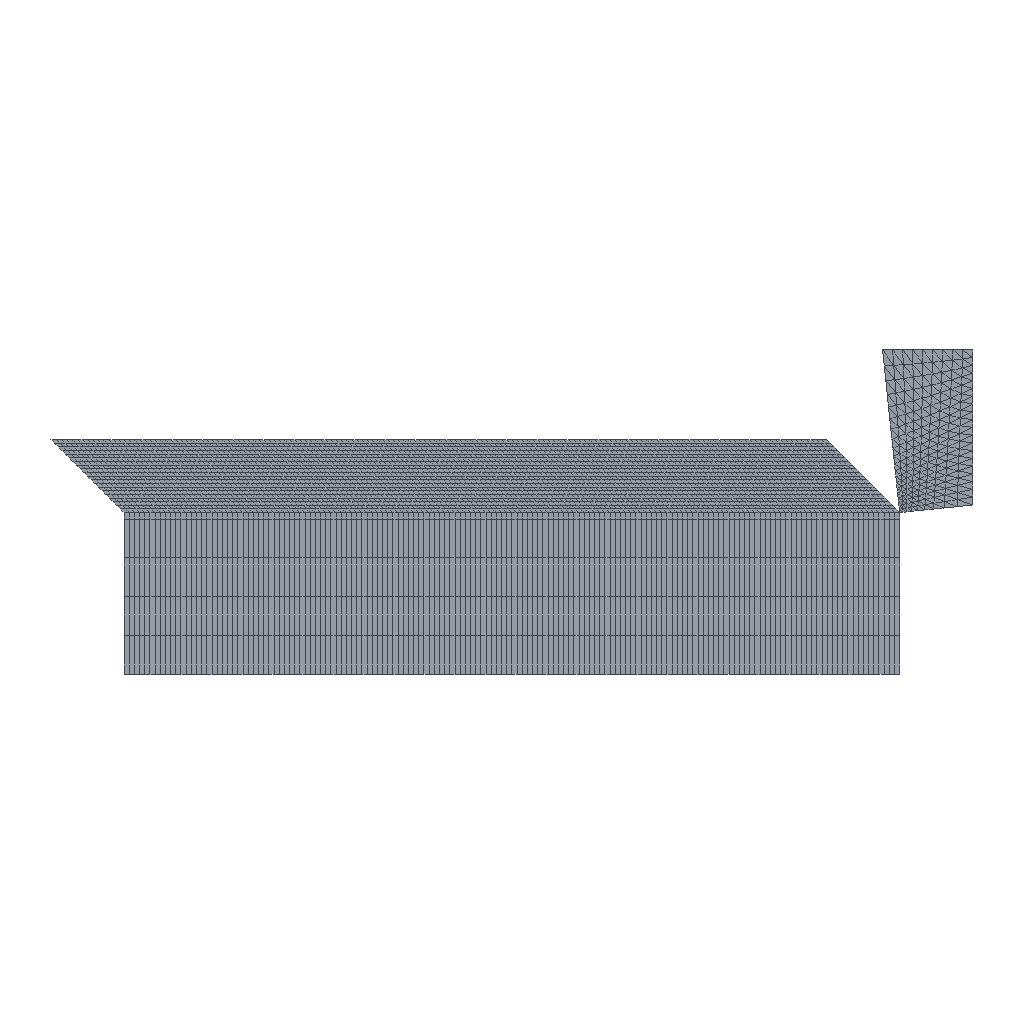Simulation study | abaqus
Set-up summary:
category,name,step,type,value,unit,region
solver,abaqus
solver,version,,,Abaqus/Explicit 2020
units,not stated in the deck,,not stated
analysis,deck,,dynamic temperature-displacement,dynamic temperature-displacement
load_step,Step-1,Step-1,dynamic temperature-displacement
load_step,requested,,,1
mesh,nodes,,,4136
mesh,elements,,,4110
element_type,CPE3T,,plane,360
element_type,CPE4RT,,plane,3750
load,load commands in deck,,count,1
bc,support commands in deck,,count,4
material,TI,,in results
material,TI-COPY,,in results
material,TI6AL4V-GAI,,in results
material,TI6AL4V-SUN,,in results
material,YG6,,in results
check,setup vs results,,match,"per instance, exact: element labels, types and connectivity; labels of the nodes the elements use; coordinates of those nodes at SINGLE_PRECISION in 2 of 2 instance(s)"
Abaqus input file, long lists of numbers shortened:
*Heading
** Job name: Job-2 Model name: Model-1-Copy
** Generated by: Abaqus/CAE 2020
*Preprint, echo=NO, model=NO, history=NO, contact=NO
**
** PARTS
**
*Part, name=Part-tool
*Node
      1, 0.05,  0.3
      2, 0.05659,  0.2373
** (208 more lines like these left out)
*Element, type=CPE3T
  1,   1,   2,  23
  2,  23,  22,   1
** (358 more lines like these left out)
*Nset, nset=Set-6, generate
   1,  210,    1
*Elset, elset=Set-6, generate
   1,  360,    1
** Section: Section-tool
*Solid Section, elset=Set-6, material=YG6
2.5,
*End Part
**
*Part, name=work
*Node
      1,          1.5, -0.2125
      2,         -1.5, -0.2125
** (3924 more lines like these left out)
*Element, type=CPE4RT
  1,    1,    9,  649,  312
  2,    9,   10,  650,  649
** (3748 more lines like these left out)
*Nset, nset=Set-4, generate
    1,  3926,     1
*Elset, elset=Set-4, generate
    1,  3750,     1
*Nset, nset=Set-12, generate
    1,  3926,     1
*Elset, elset=Set-12
    1,    2,    3,    4,    5,    6,    7,    8,    9,   10,   11,   12,   13,   14,   15,   16
   17,   18,   19,   20,   21,   22,   23,   24,   25,   26,   27,   28,   29,   30,   31,   32
** (223 more lines like these left out)
*Nset, nset=Set-13
   1,   2,   5,   6,   9,  10,  11,  12,  13,  14,  15,  16,  17,  18,  19,  20
  21,  22,  23,  24,  25,  26,  27,  28,  29,  30,  31,  32,  33,  34,  35,  36
** (17 more lines like these left out)
*Elset, elset=Set-13, generate
 601,  750,    1
** Section: ti
*Solid Section, elset=Set-12, material=ti
,
** Section: middle
*Solid Section, elset=Set-13, material=ti-Copy
,
*End Part
**
**
** ASSEMBLY
**
*Assembly, name=Assembly
**
*Instance, name=Part-tool-1, part=Part-tool
    1.384,     0.1423,           0.
*End Instance
**
*Instance, name=work-1, part=work
*End Instance
**
*Node
      1,   1.784,   0.4423,           0.
*Nset, nset=Set-9, instance=work-1, generate
    1,  3926,     1
*Elset, elset=Set-9, instance=work-1, generate
    1,  3750,     1
*Nset, nset=Set-10, instance=Part-tool-1, generate
   1,  210,    1
*Elset, elset=Set-10, instance=Part-tool-1, generate
   1,  360,    1
*Nset, nset=Set-11, instance=work-1
   2,   3,   4, 158, 159, 160, 161, 162, 163, 164, 165, 166, 167, 168, 169, 170
 171, 172, 173, 174, 175, 176, 177, 178, 179, 180, 181, 182, 183, 184, 185, 186
** (8 more lines like these left out)
*Elset, elset=Set-11, instance=work-1
 150, 300, 450, 451, 452, 453, 454, 455, 456, 457, 458, 459, 460, 461, 462, 463
 464, 465, 466, 467, 468, 469, 470, 471, 472, 473, 474, 475, 476, 477, 478, 479
** (8 more lines like these left out)
*Nset, nset=Set-RP
 1,
*Nset, nset=b_Set-7, instance=Part-tool-1, generate
   1,  210,    1
*Elset, elset=b_Set-7, instance=Part-tool-1, generate
   1,  360,    1
*Nset, nset=s_Set-12, instance=work-1
    1,    2,    5,    6,    7,    8,    9,   10,   11,   12,   13,   14,   15,   16,   17,   18
   19,   20,   21,   22,   23,   24,   25,   26,   27,   28,   29,   30,   31,   32,   33,   34
** (206 more lines like these left out)
*Elset, elset=s_Set-12, instance=work-1, generate
  601,  3750,     1
*Nset, nset=s_Set-13, instance=work-1
    1,    2,    5,    6,    7,    8,    9,   10,   11,   12,   13,   14,   15,   16,   17,   18
   19,   20,   21,   22,   23,   24,   25,   26,   27,   28,   29,   30,   31,   32,   33,   34
** (206 more lines like these left out)
*Elset, elset=s_Set-13, instance=work-1, generate
  601,  3750,     1
*Nset, nset=_PickedSet38, internal
 1,
*Elset, elset=_Surf-8_S2, internal, instance=work-1, generate
  750,  3750,   150
*Elset, elset=_Surf-8_S1, internal, instance=work-1, generate
 751,  900,    1
*Elset, elset=_Surf-8_S4, internal, instance=work-1, generate
  751,  3601,   150
*Surface, type=ELEMENT, name=Surf-8
_Surf-8_S2, S2
_Surf-8_S1, S1
_Surf-8_S4, S4
*Elset, elset=_m_Surf-7_S1, internal, instance=Part-tool-1, generate
  1,  39,   2
*Elset, elset=_m_Surf-7_S2, internal, instance=Part-tool-1
   2,  39,  42,  79,  82, 119, 122, 159, 162, 199, 202, 239, 242, 279, 282, 319
 322, 359
*Surface, type=ELEMENT, name=m_Surf-7
_m_Surf-7_S1, S1
_m_Surf-7_S2, S2
*Surface, type=NODE, name=s_Set-13_CNS_, internal
s_Set-13, 1.
** Constraint: Constraint-1
*Rigid Body, ref node=_PickedSet38, elset=b_Set-7, position=CENTER OF MASS
*End Assembly
**
** MATERIALS
**
*Material, name=TI6AL4V-gai
*Conductivity
  5.44, 20.
   6.7,100.
  8.79,200.
 10.47,300.
 12.56,400.
 14.24,500.
 15.49,600.
*Damage Initiation, criterion=JOHNSON COOK
 -0.09,  0.25, -0.48, 0.014,  3.87, 1630.,   25.,    1.
*Damage Evolution, type=DISPLACEMENT
 0.1,
*Density
 4.44e-09,
*Elastic
105000., 0.31
*Expansion
 9.4e-06,100.
 9.5e-06,200.
 9.6e-06,300.
 9.7e-06,400.
 9.9e-06,500.
   1e-05,600.
*Inelastic Heat Fraction
         0.9,
*Plastic, hardening=JOHNSON COOK
875.,  793., 0.386,  0.71, 1630.,   25.
*Rate Dependent, type=JOHNSON COOK
 0.01,1.
*Specific Heat
 5.65e+08, 20.
 6.78e+08,100.
 6.91e+08,200.
 7.03e+08,300.
 7.41e+08,400.
 7.54e+08,500.
 8.79e+08,600.
*Material, name=TI6AL4V-sun
*Conductivity
  5.44, 20.
   6.7,100.
  8.79,200.
 10.47,300.
 12.56,400.
 14.24,500.
 15.49,600.
*Damage Initiation, criterion=JOHNSON COOK
 -0.09,  0.25, -0.48, 0.014,  3.87, 1630.,   25.,    1.
*Damage Evolution, type=DISPLACEMENT
 0.15,
*Density
 4.44e-09,
*Elastic
105000., 0.31
*Expansion
 9.4e-06,100.
 9.5e-06,200.
 9.6e-06,300.
 9.7e-06,400.
 9.9e-06,500.
   1e-05,600.
*Inelastic Heat Fraction
         0.9,
*Plastic, hardening=JOHNSON COOK
875.,  793., 0.386,  0.71, 1630.,   25.
*Rate Dependent, type=JOHNSON COOK
 0.01,1.
*Specific Heat
 5.65e+08, 20.
 6.78e+08,100.
 6.91e+08,200.
 7.03e+08,300.
 7.41e+08,400.
 7.54e+08,500.
 8.79e+08,600.
*Material, name=YG6
*Conductivity
 79.6,
*Density
 1.485e-08,
*Elastic
640000., 0.22
*Expansion
 4.7e-06,
*Inelastic Heat Fraction
         0.9,
*Specific Heat
 1.76e+08,
*Material, name=ti
*Conductivity
  7.5, 20.
  8.7,200.
 11.8,500.
*Damage Initiation, criterion=JOHNSON COOK
 -0.09,  0.25,  -0.5, 0.014,  3.87, 1650.,   25.,    1.
*Damage Evolution, type=DISPLACEMENT
 0.1,
*Density
 4.44e-09,
*Elastic
108000., 0.33
*Expansion
 9.1e-06, 20.
 9.2e-06,250.
 9.7e-06,500.
*Inelastic Heat Fraction
         0.9,
*Plastic, hardening=JOHNSON COOK
860., 683., 0.47,   1.,1650.,  25.
*Rate Dependent, type=JOHNSON COOK
 0.035,1.
*Specific Heat
 5.263e+08,
*Material, name=ti-Copy
*Conductivity
  7.5, 20.
  8.7,200.
 11.8,500.
*Damage Initiation, criterion=JOHNSON COOK
 -0.09,  0.25,  -0.5, 0.014,  3.87, 1650.,   25.,    1.
*Damage Evolution, type=DISPLACEMENT
 0.04,
*Density
 4.44e-09,
*Elastic
108000., 0.33
*Expansion
 9.1e-06, 20.
 9.2e-06,250.
 9.7e-06,500.
*Inelastic Heat Fraction
         0.9,
*Plastic, hardening=JOHNSON COOK
860., 683., 0.47,   1.,1650.,  25.
*Rate Dependent, type=JOHNSON COOK
 0.035,1.
*Specific Heat
 5.263e+08,
**
** INTERACTION PROPERTIES
**
*Surface Interaction, name=IntProp-1
*Friction
 0.1,
*Surface Behavior, pressure-overclosure=HARD
*Surface Interaction, name=zijie
*Friction
 0.5,
*Surface Behavior, pressure-overclosure=HARD
**
** BOUNDARY CONDITIONS
**
** Name: BC-1 Type: 对称/反对称/完全固定
*Boundary
Set-11, ENCASTRE
**
** PREDEFINED FIELDS
**
** Name: Predefined Field-1   Type: Temperature
*Initial Conditions, type=TEMPERATURE
Set-9, 20.
** Name: Predefined Field-2   Type: Temperature
*Initial Conditions, type=TEMPERATURE
Set-10, 20.
** ----------------------------------------------------------------
**
** STEP: Step-1
**
*Step, name=Step-1, nlgeom=YES
*Dynamic Temperature-displacement, Explicit
, 0.001
*Bulk Viscosity
0.06, 1.2
** Mass Scaling: Semi-Automatic
**               Whole Model
*Fixed Mass Scaling, factor=200.
**
** BOUNDARY CONDITIONS
**
** Name: BC-2 Type: 速度/角速度
*Boundary, type=VELOCITY
Set-RP, 1, 1, -1666.
Set-RP, 2, 2
Set-RP, 6, 6
*Adaptive Mesh Controls, name=Ada-1, curvature refinement=5.
0.5, 0., 0.5
**
** INTERACTIONS
**
** Interaction: Int-1
*Contact Pair, interaction=IntProp-1, mechanical constraint=KINEMATIC, cpset=Int-1
m_Surf-7, s_Set-13_CNS_
** Interaction: Int-2
*Contact, op=NEW
*Contact Inclusions, ALL EXTERIOR
*Contact Property Assignment
 ,  , zijie
**
** OUTPUT REQUESTS
**
*Restart, write, number interval=1, time marks=NO
**
** FIELD OUTPUT: F-Output-1
**
*Output, field, number interval=100
*Node Output
A, NT, RF, RFL, U, V
*Element Output, directions=YES
E, EVF, HFL, LE, MISES, PE, PEEQ, PEEQVAVG, PEVAVG, S, STATUS, SVAVG, TEMP
*Contact Output
CSTRESS,
**
** HISTORY OUTPUT: H-Output-1
**
*Output, history, time interval=5e-07
*Node Output, nset=Set-RP
RF1, RF2, RF3
*End Step
Results summary:
result,step,Step-1,completed,increments=124695 time=0.001/0.001
result,analysis,,,"dynamic temperature-displacement, explict"
result,last_loadstep,,,1
result,primary field,,,"U, NT11"
result,reaction total,,FX,-3.478,model units
result,reaction total,,FY,7.793,model units
result,reaction total,,FZ,0.0,model units